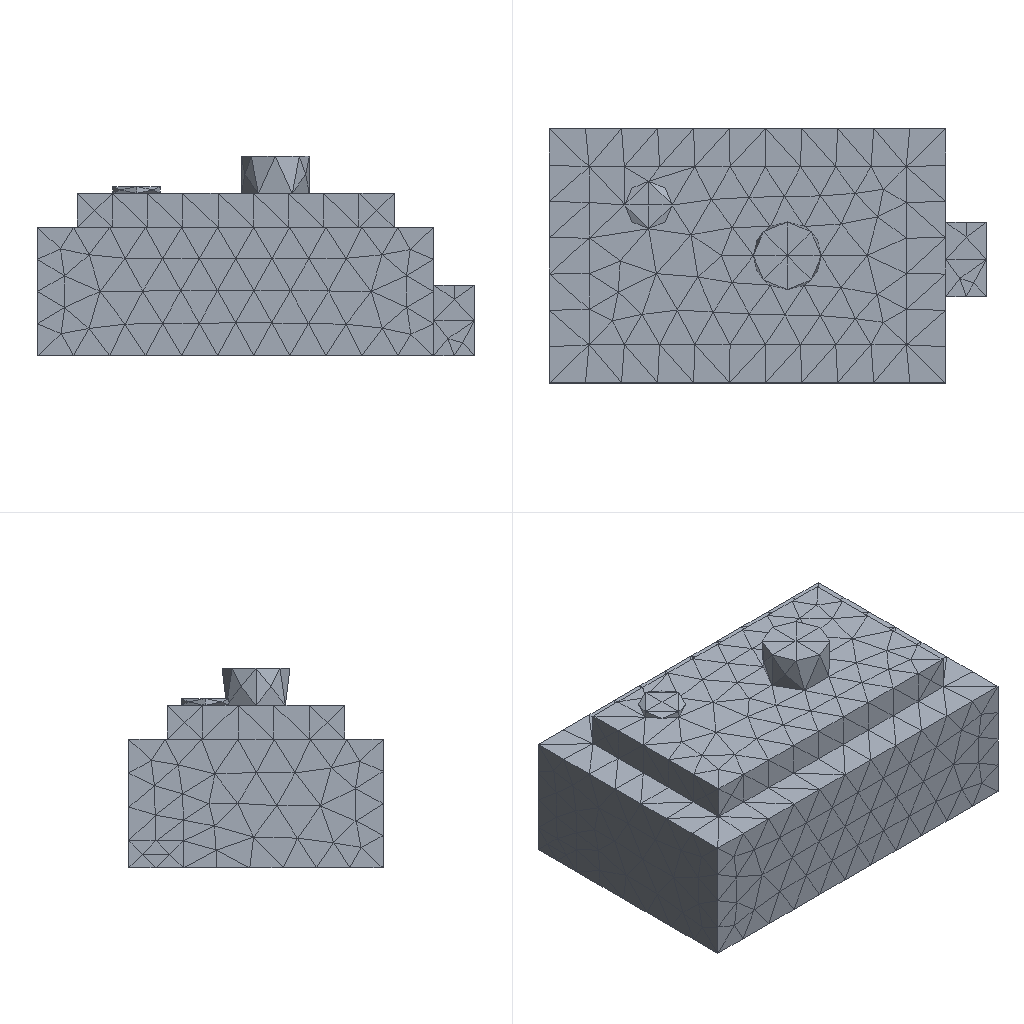Simulation study | ansys mapdl
Set-up summary:
category,name,step,type,value,unit,region
solver,ansys_mapdl
units,mm-N-s-tonne (MPa),,inferred,E=210000 density=
analysis,model,,static
mesh,nodes,,,4919
mesh,elements,,,2975
element_type,SOLID187,,,2975
material,mat 1,,E,210000
material,mat 1,,nu,0.3
load,,model,body load temp,,,all
load,,model,force,"1000 [dir=(0, 0, -1) n=113]",,node list
bc,,model,fixed,"[dofs=UX,UY,UZ n=5484]",,node list
Ansys APDL input file, long lists of numbers shortened:
/COM,ANSYS RELEASE 2026 R1           BUILD 26.1      UP20260202       09:10:51
/PREP7
/NOPR
/TITLE,2
ANTYPE, 0
*IF,_CDRDOFF,EQ,1,THEN     !if solid model was read in
_CDRDOFF=             !reset flag, numoffs already performed
*ELSE              !offset database for the following FE model
NUMOFF,NODE,     4919
NUMOFF,ELEM,     2975
NUMOFF,MAT ,        1
NUMOFF,TYPE,        1
*ENDIF
*SET,_RETURN ,  0.
*SET,_STATUS ,  0.
*SET,_UIQR   ,  113.
*SET,__FLOATPARAMETER__,  4919.
DOF,DELETE
ETBLOCK,        1,        1
(2i9,19a9)
        1      187        0        0        0        0        0        0        0        0        0        0        0        0        0        0        0        0        0        0        0
       -1
NBLOCK,6,SOLID,      4919,      4919
(3i9,6e21.13e3)
        1        0        0-4.2475000000000E+001 3.7500000000000E+001 8.0000000000000E+000
! (4918 more lines like these left out)
N,UNBL,LOC,       -1,
EBLOCK,19,SOLID,      2975,      2975
(19i10)
         1         1         1         1         0         0         0         0        10         0         1      1807      1808      1809      1810      2101      2102      2103      2104
! (5949 more lines like these left out)
        -1
MPTEMP,UNBL, 1, 1,  0.    ,
MPDATA,UNBL, 1,EX  ,       1, 1,  210000.000    ,
MPTEMP,UNBL, 1, 1,  0.    ,
MPDATA,UNBL, 1,NUXY,       1, 1, 0.3    ,
MPTEMP,UNBL, 1, 1,  0.    ,
MPDATA,UNBL, 1,PRXY,       1, 1, 0.3    ,
EXTOPT,ATTR,      0,      0,      0
EXTOPT,ESIZE,  0,  0.
EXTOPT,ACLEAR,      0
TREF,  0.
IRLF,  0
BFUNIF,TEMP,_TINY
ACEL,  0.    ,  0.    ,  0.
OMEGA,  0.    ,  0.    ,  0.
DOMEGA,  0.    ,  0.    ,  0.
CGLOC,  0.    ,  0.    ,  0.
CGOMEGA,  0.    ,  0.    ,  0.
DCGOMG,  0.    ,  0.    ,  0.
KUSE,     0
TIME,  0.
ALPHAD,  0.
BETAD,  0.
DMPRAT,  0.
DMPSTR,  0.
CRPLIM, 0.1    ,   0
CRPLIM,  0.    ,   1
NCNV,     0, 1.000000000E+12,     0,  0.    ,  0.
NEQIT,     0
ERESX,DEFA
DBLOCK,      5484
(i9,a6,2(pg16.9))
        1  UX    0.00000000      0.00000000
! (5483 more lines like these left out)
       -1
FBLOCK,       113
(i9,a6,2(pg16.9))
      870  FZ   -8.84955752      0.00000000
! (112 more lines like these left out)
       -1
/GO
FINISH
Results summary:
result,analysis_type_db,,,static,unstated
result,n_sets,,,1,unstated
result,load_steps[0].set,load_step=1,,1,unstated
result,load_steps[0].substep,load_step=1,,1,unstated
result,load_steps[0].time,load_step=1,,1,unstated
result,load_steps[0].freq,load_step=1,,1,unstated
result,load_steps[0].max_usum,load_step=1,,0.0002205,unstated
result,load_steps[0].max_seqv,load_step=1,,13.948,unstated
result,load_steps[0].reaction_sum.FX,load_step=1,,-5.89174e-12,unstated
result,load_steps[0].reaction_sum.FY,load_step=1,,-1.33741e-11,unstated
result,load_steps[0].reaction_sum.FZ,load_step=1,,1000,unstated
result,load_steps[0].reaction_sum.MX,load_step=1,,0,unstated
result,load_steps[0].reaction_sum.MY,load_step=1,,0,unstated
result,load_steps[0].reaction_sum.MZ,load_step=1,,0,unstated
result,convergence,,,results present for all listed sets,unstated